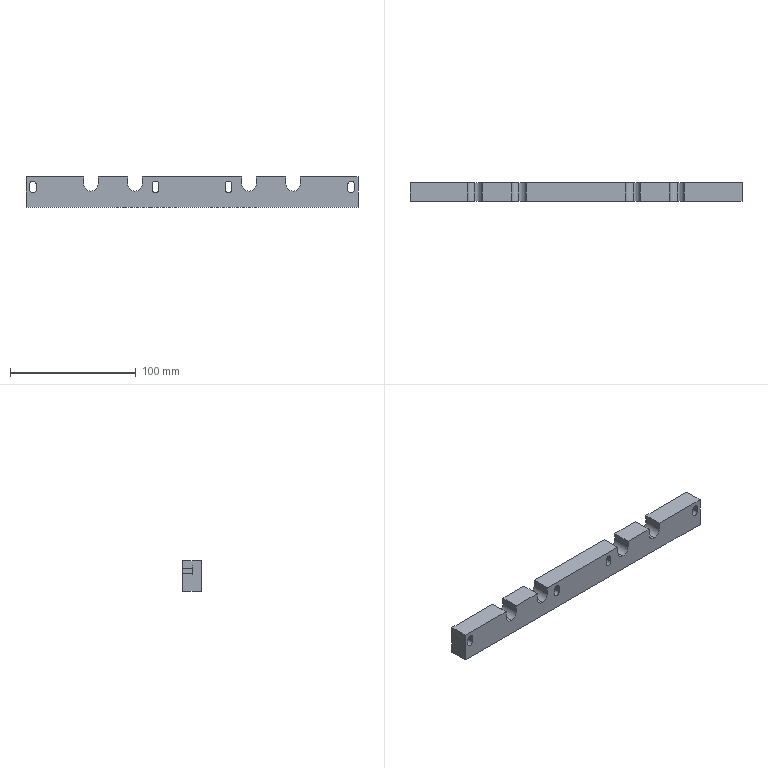Part | 1 solid | 70 faces | box 263.5 x 15 x 24 mm | volume 82979 mm3 | plane 38 | cylinder 32 | commonest cylinder face diameters 5.2 x12 10 x12 11.5 x8